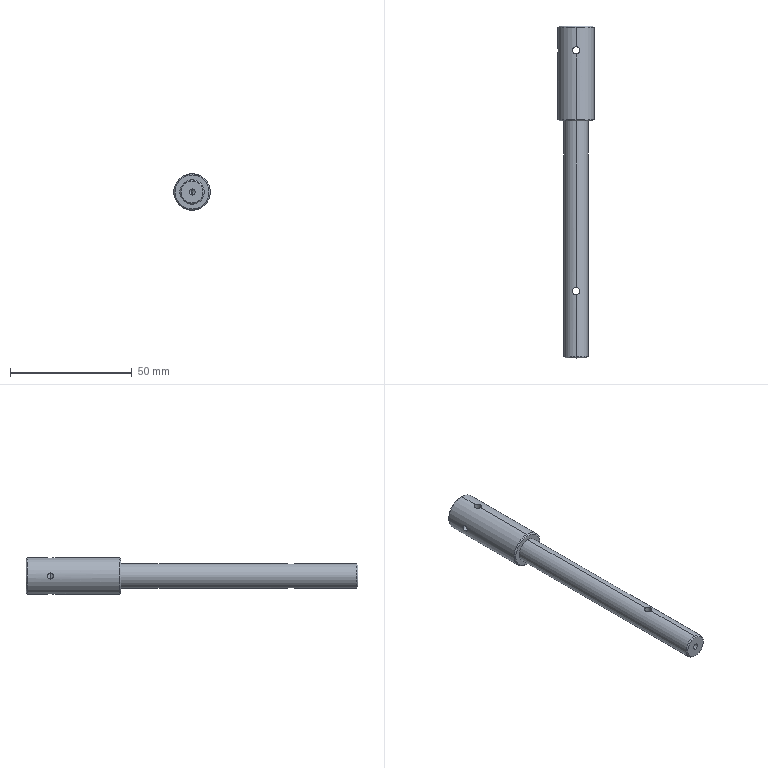Part | SolidWorks | features 3DProfileFeature 3, HoleWzd 3, ICE 2, Chamfer 1, Revolution 1 | 1 solid | 27 faces | box 15 x 136.5 x 15 mm | volume 14219 mm3 | cylinder 14 | cone 10 | plane 3 | commonest cylinder face diameters 2.5 x4 3 x4 3.3 x2 10 x2 15 x2
STEP:
#1=CARTESIAN_POINT('',(0.,-110.5,-5.));
#2=VERTEX_POINT('',#1);
#3=CARTESIAN_POINT('',(-1.5,-109.,-4.77));
#4=VERTEX_POINT('',#3);
#5=CARTESIAN_POINT('',(0.,-110.5,-5.));
#6=CARTESIAN_POINT('',(-0.09847,-110.5,-5.));
#7=CARTESIAN_POINT('',(-0.1985,-110.49,-4.997));
#8=CARTESIAN_POINT('',(-0.3913,-110.451,-4.986));
#9=CARTESIAN_POINT('',(-0.4851,-110.423,-4.977));
#10=CARTESIAN_POINT('',(-0.7586,-110.309,-4.946));
#11=CARTESIAN_POINT('',(-0.9231,-110.198,-4.916));
#12=CARTESIAN_POINT('',(-1.131,-109.991,-4.871));
#13=CARTESIAN_POINT('',(-1.192,-109.916,-4.856));
#14=CARTESIAN_POINT('',(-1.301,-109.753,-4.828));
#15=CARTESIAN_POINT('',(-1.348,-109.666,-4.815));
#16=CARTESIAN_POINT('',(-1.423,-109.485,-4.793));
#17=CARTESIAN_POINT('',(-1.451,-109.391,-4.785));
#18=CARTESIAN_POINT('',(-1.49,-109.198,-4.773));
#19=CARTESIAN_POINT('',(-1.5,-109.098,-4.77));
#20=CARTESIAN_POINT('',(-1.5,-109.,-4.77));
#21=B_SPLINE_CURVE_WITH_KNOTS('',3,(#5,#6,#7,#8,#9,#10,#11,#12,#13,#14,#15,#16,#17,#18,#19,#20),.UNSPECIFIED.,.F.,.F.,(4,2,2,2,2,2,2,4),(0.002359,0.002654,0.002949,0.003538,0.003833,0.004127,0.004422,0.004717),.UNSPECIFIED.);
#22=EDGE_CURVE('',#2,#4,#21,.T.);
#23=ORIENTED_EDGE('',*,*,#22,.T.);
#24=CARTESIAN_POINT('',(-1.5,-109.,4.77));
#25=VERTEX_POINT('',#24);
#26=CARTESIAN_POINT('',(-1.5,-109.,-8.));
#27=DIRECTION('',(0.,0.,1.));
#28=VECTOR('',#27,1000.);
#29=LINE('',#26,#28);
#30=EDGE_CURVE('',#4,#25,#29,.T.);
#31=ORIENTED_EDGE('',*,*,#30,.T.);
#32=CARTESIAN_POINT('',(0.,-110.5,5.));
#33=VERTEX_POINT('',#32);
#34=CARTESIAN_POINT('',(-1.5,-109.,4.77));
#35=CARTESIAN_POINT('',(-1.5,-109.099,4.77));
#36=CARTESIAN_POINT('',(-1.49,-109.197,4.773));
#37=CARTESIAN_POINT('',(-1.452,-109.39,4.785));
#38=CARTESIAN_POINT('',(-1.423,-109.486,4.794));
#39=CARTESIAN_POINT('',(-1.31,-109.757,4.826));
#40=CARTESIAN_POINT('',(-1.198,-109.923,4.856));
#41=CARTESIAN_POINT('',(-0.9923,-110.129,4.901));
#42=CARTESIAN_POINT('',(-0.9158,-110.192,4.916));
#43=CARTESIAN_POINT('',(-0.7532,-110.301,4.944));
#44=CARTESIAN_POINT('',(-0.6674,-110.347,4.956));
#45=CARTESIAN_POINT('',(-0.4865,-110.422,4.977));
#46=CARTESIAN_POINT('',(-0.3907,-110.452,4.986));
#47=CARTESIAN_POINT('',(-0.1978,-110.49,4.997));
#48=CARTESIAN_POINT('',(-0.0997,-110.5,5.));
#49=CARTESIAN_POINT('',(0.,-110.5,5.));
#50=B_SPLINE_CURVE_WITH_KNOTS('',3,(#34,#35,#36,#37,#38,#39,#40,#41,#42,#43,#44,#45,#46,#47,#48,#49),.UNSPECIFIED.,.F.,.F.,(4,2,2,2,2,2,2,4),(0.007075,0.00737,0.007664,0.008254,0.008549,0.008843,0.009138,0.009433),.UNSPECIFIED.);
#51=EDGE_CURVE('',#25,#33,#50,.T.);
#52=ORIENTED_EDGE('',*,*,#51,.T.);
#53=CARTESIAN_POINT('',(1.5,-109.,4.77));
#54=VERTEX_POINT('',#53);
#55=CARTESIAN_POINT('',(0.,-110.5,5.));
#56=CARTESIAN_POINT('',(0.09976,-110.5,5.));
#57=CARTESIAN_POINT('',(0.1977,-110.49,4.997));
#58=CARTESIAN_POINT('',(0.3903,-110.452,4.986));
#59=CARTESIAN_POINT('',(0.4859,-110.423,4.977));
#60=CARTESIAN_POINT('',(0.6674,-110.347,4.956));
#61=CARTESIAN_POINT('',(0.7534,-110.301,4.944));
#62=CARTESIAN_POINT('',(0.916,-110.192,4.916));
#63=CARTESIAN_POINT('',(0.9926,-110.129,4.901));
#64=CARTESIAN_POINT('',(1.199,-109.922,4.856));
#65=CARTESIAN_POINT('',(1.31,-109.756,4.826));
#66=CARTESIAN_POINT('',(1.46,-109.395,4.783));
#67=CARTESIAN_POINT('',(1.5,-109.197,4.77));
#68=CARTESIAN_POINT('',(1.5,-109.,4.77));
#69=B_SPLINE_CURVE_WITH_KNOTS('',3,(#55,#56,#57,#58,#59,#60,#61,#62,#63,#64,#65,#66,#67,#68),.UNSPECIFIED.,.F.,.F.,(4,2,2,2,2,2,4),(0.,0.0002949,0.0005898,0.0008847,0.00118,0.001769,0.002359),.UNSPECIFIED.);
#70=EDGE_CURVE('',#33,#54,#69,.T.);
#71=ORIENTED_EDGE('',*,*,#70,.T.);
#72=CARTESIAN_POINT('',(1.5,-109.,-4.77));
#73=VERTEX_POINT('',#72);
#74=CARTESIAN_POINT('',(1.5,-109.,-8.));
#75=DIRECTION('',(0.,0.,1.));
#76=VECTOR('',#75,1000.);
#77=LINE('',#74,#76);
#78=EDGE_CURVE('',#73,#54,#77,.T.);
#79=ORIENTED_EDGE('',*,*,#78,.F.);
#80=CARTESIAN_POINT('',(1.5,-109.,-4.77));
#81=CARTESIAN_POINT('',(1.5,-109.1,-4.77));
#82=CARTESIAN_POINT('',(1.49,-109.198,-4.773));
#83=CARTESIAN_POINT('',(1.452,-109.39,-4.785));
#84=CARTESIAN_POINT('',(1.423,-109.486,-4.794));
#85=CARTESIAN_POINT('',(1.347,-109.667,-4.815));
#86=CARTESIAN_POINT('',(1.301,-109.753,-4.828));
#87=CARTESIAN_POINT('',(1.192,-109.916,-4.856));
#88=CARTESIAN_POINT('',(1.129,-109.992,-4.871));
#89=CARTESIAN_POINT('',(0.9226,-110.199,-4.916));
#90=CARTESIAN_POINT('',(0.7561,-110.31,-4.946));
#91=CARTESIAN_POINT('',(0.3953,-110.46,-4.988));
#92=CARTESIAN_POINT('',(0.197,-110.5,-5.));
#93=CARTESIAN_POINT('',(0.,-110.5,-5.));
#94=B_SPLINE_CURVE_WITH_KNOTS('',3,(#80,#81,#82,#83,#84,#85,#86,#87,#88,#89,#90,#91,#92,#93),.UNSPECIFIED.,.F.,.F.,(4,2,2,2,2,2,4),(0.,0.0002949,0.0005898,0.0008847,0.00118,0.001769,0.002359),.UNSPECIFIED.);
#95=EDGE_CURVE('',#73,#2,#94,.T.);
#96=ORIENTED_EDGE('',*,*,#95,.T.);
#97=EDGE_LOOP('',(#23,#31,#52,#71,#79,#96));
#98=FACE_OUTER_BOUND('',#97,.T.);
#99=CARTESIAN_POINT('',(0.,-109.,-8.));
#100=DIRECTION('',(0.,0.,1.));
#101=DIRECTION('',(1.,0.,0.));
#102=AXIS2_PLACEMENT_3D('',#99,#100,#101);
#103=CYLINDRICAL_SURFACE('',#102,1.5);
#104=ADVANCED_FACE('',(#98),#103,.F.);
#105=CARTESIAN_POINT('',(-1.5,-10.,-1.25));
#106=VERTEX_POINT('',#105);
#107=CARTESIAN_POINT('',(-1.5,-10.,1.25));
#108=VERTEX_POINT('',#107);
#109=CARTESIAN_POINT('',(-1.5,-10.,-1.25));
#110=CARTESIAN_POINT('',(-1.5,-10.175,-1.25));
#111=CARTESIAN_POINT('',(-1.468,-10.349,-1.212));
#112=CARTESIAN_POINT('',(-1.36,-10.654,-1.078));
#113=CARTESIAN_POINT('',(-1.285,-10.786,-0.9844));
#114=CARTESIAN_POINT('',(-1.125,-11.002,-0.7635));
#115=CARTESIAN_POINT('',(-1.037,-11.088,-0.6353));
#116=CARTESIAN_POINT('',(-0.9263,-11.181,-0.4177));
#117=CARTESIAN_POINT('',(-0.8924,-11.206,-0.3392));
#118=CARTESIAN_POINT('',(-0.8438,-11.241,-0.1749));
#119=CARTESIAN_POINT('',(-0.8291,-11.25,-0.08668));
#120=CARTESIAN_POINT('',(-0.8292,-11.25,0.08724));
#121=CARTESIAN_POINT('',(-0.8439,-11.24,0.1754));
#122=CARTESIAN_POINT('',(-0.8925,-11.206,0.3393));
#123=CARTESIAN_POINT('',(-0.9262,-11.181,0.4175));
#124=CARTESIAN_POINT('',(-1.037,-11.088,0.636));
#125=CARTESIAN_POINT('',(-1.125,-11.001,0.7639));
#126=CARTESIAN_POINT('',(-1.245,-10.839,0.9296));
#127=CARTESIAN_POINT('',(-1.283,-10.78,0.98));
#128=CARTESIAN_POINT('',(-1.354,-10.649,1.071));
#129=CARTESIAN_POINT('',(-1.387,-10.577,1.112));
#130=CARTESIAN_POINT('',(-1.468,-10.35,1.211));
#131=CARTESIAN_POINT('',(-1.5,-10.177,1.25));
#132=CARTESIAN_POINT('',(-1.5,-10.,1.25));
#133=B_SPLINE_CURVE_WITH_KNOTS('',3,(#109,#110,#111,#112,#113,#114,#115,#116,#117,#118,#119,#120,#121,#122,#123,#124,#125,#126,#127,#128,#129,#130,#131,#132),.UNSPECIFIED.,.F.,.F.,(4,2,2,2,2,2,2,2,2,2,2,4),(0.004174,0.004695,0.005216,0.005737,0.005998,0.006258,0.006519,0.006779,0.0073,0.007561,0.007821,0.008342),.UNSPECIFIED.);
#134=EDGE_CURVE('',#106,#108,#133,.T.);
#135=ORIENTED_EDGE('',*,*,#134,.F.);
#136=CARTESIAN_POINT('',(-7.395,-10.,-1.25));
#137=VERTEX_POINT('',#136);
#138=CARTESIAN_POINT('',(-7.5,-10.,-1.25));
#139=DIRECTION('',(-1.,0.,0.));
#140=VECTOR('',#139,1000.);
#141=LINE('',#138,#140);
#142=EDGE_CURVE('',#106,#137,#141,.T.);
#143=ORIENTED_EDGE('',*,*,#142,.T.);
#144=CARTESIAN_POINT('',(-7.395,-10.,1.25));
#145=VERTEX_POINT('',#144);
#146=CARTESIAN_POINT('',(-7.395,-10.,-1.25));
#147=CARTESIAN_POINT('',(-7.395,-10.163,-1.25));
#148=CARTESIAN_POINT('',(-7.401,-10.328,-1.217));
#149=CARTESIAN_POINT('',(-7.42,-10.629,-1.092));
#150=CARTESIAN_POINT('',(-7.434,-10.768,-0.9996));
#151=CARTESIAN_POINT('',(-7.455,-10.941,-0.8269));
#152=CARTESIAN_POINT('',(-7.461,-10.994,-0.7627));
#153=CARTESIAN_POINT('',(-7.474,-11.084,-0.6272));
#154=CARTESIAN_POINT('',(-7.48,-11.123,-0.5555));
#155=CARTESIAN_POINT('',(-7.494,-11.217,-0.3283));
#156=CARTESIAN_POINT('',(-7.5,-11.25,-0.1659));
#157=CARTESIAN_POINT('',(-7.5,-11.25,0.1644));
#158=CARTESIAN_POINT('',(-7.494,-11.217,0.3271));
#159=CARTESIAN_POINT('',(-7.475,-11.092,0.6295));
#160=CARTESIAN_POINT('',(-7.461,-10.999,0.7682));
#161=CARTESIAN_POINT('',(-7.434,-10.77,0.9984));
#162=CARTESIAN_POINT('',(-7.42,-10.63,1.092));
#163=CARTESIAN_POINT('',(-7.401,-10.33,1.217));
#164=CARTESIAN_POINT('',(-7.395,-10.165,1.25));
#165=CARTESIAN_POINT('',(-7.395,-10.,1.25));
#166=B_SPLINE_CURVE_WITH_KNOTS('',3,(#146,#147,#148,#149,#150,#151,#152,#153,#154,#155,#156,#157,#158,#159,#160,#161,#162,#163,#164,#165),.UNSPECIFIED.,.F.,.F.,(4,2,2,2,2,2,2,2,2,4),(0.003915,0.004404,0.004893,0.005138,0.005383,0.005872,0.006361,0.00685,0.00734,0.007829),.UNSPECIFIED.);
#167=EDGE_CURVE('',#137,#145,#166,.T.);
#168=ORIENTED_EDGE('',*,*,#167,.T.);
#169=CARTESIAN_POINT('',(-7.5,-10.,1.25));
#170=DIRECTION('',(-1.,0.,0.));
#171=VECTOR('',#170,1000.);
#172=LINE('',#169,#171);
#173=EDGE_CURVE('',#108,#145,#172,.T.);
#174=ORIENTED_EDGE('',*,*,#173,.F.);
#175=EDGE_LOOP('',(#135,#143,#168,#174));
#176=FACE_OUTER_BOUND('',#175,.T.);
#177=CARTESIAN_POINT('',(-7.5,-10.,0.));
#178=DIRECTION('',(-1.,0.,0.));
#179=DIRECTION('',(0.,0.,1.));
#180=AXIS2_PLACEMENT_3D('',#177,#178,#179);
#181=CYLINDRICAL_SURFACE('',#180,1.25);
#182=ADVANCED_FACE('',(#176),#181,.F.);
#183=CARTESIAN_POINT('',(0.,-136.5,-4.5));
#184=VERTEX_POINT('',#183);
#185=CARTESIAN_POINT('',(0.,-136.5,4.5));
#186=VERTEX_POINT('',#185);
#187=CARTESIAN_POINT('',(0.,-136.5,0.));
#188=DIRECTION('',(0.,-1.,0.));
#189=DIRECTION('',(0.,0.,-1.));
#190=AXIS2_PLACEMENT_3D('',#187,#188,#189);
#191=CIRCLE('',#190,4.5);
#192=EDGE_CURVE('',#184,#186,#191,.T.);
#193=ORIENTED_EDGE('',*,*,#192,.F.);
#194=CARTESIAN_POINT('',(0.,-136.,-5.));
#195=VERTEX_POINT('',#194);
#196=CARTESIAN_POINT('',(0.,-136.,-5.));
#197=DIRECTION('',(0.,0.7071,-0.7071));
#198=VECTOR('',#197,1000.);
#199=LINE('',#196,#198);
#200=EDGE_CURVE('',#184,#195,#199,.T.);
#201=ORIENTED_EDGE('',*,*,#200,.T.);
#202=CARTESIAN_POINT('',(0.,-136.,5.));
#203=VERTEX_POINT('',#202);
#204=CARTESIAN_POINT('',(0.,-136.,0.));
#205=DIRECTION('',(0.,1.,0.));
#206=DIRECTION('',(0.,0.,-1.));
#207=AXIS2_PLACEMENT_3D('',#204,#205,#206);
#208=CIRCLE('',#207,5.);
#209=EDGE_CURVE('',#203,#195,#208,.T.);
#210=ORIENTED_EDGE('',*,*,#209,.F.);
#211=CARTESIAN_POINT('',(0.,-136.,5.));
#212=DIRECTION('',(0.,0.7071,0.7071));
#213=VECTOR('',#212,1000.);
#214=LINE('',#211,#213);
#215=EDGE_CURVE('',#186,#203,#214,.T.);
#216=ORIENTED_EDGE('',*,*,#215,.F.);
#217=EDGE_LOOP('',(#193,#201,#210,#216));
#218=FACE_OUTER_BOUND('',#217,.T.);
#219=CARTESIAN_POINT('',(0.,-136.,0.));
#220=DIRECTION('',(0.,1.,0.));
#221=DIRECTION('',(0.,0.,1.));
#222=AXIS2_PLACEMENT_3D('',#219,#220,#221);
#223=CONICAL_SURFACE('',#222,5.,0.7854);
#224=ADVANCED_FACE('',(#218),#223,.T.);
#225=CARTESIAN_POINT('',(0.,-39.,-7.));
#226=VERTEX_POINT('',#225);
#227=CARTESIAN_POINT('',(0.,-39.,7.));
#228=VERTEX_POINT('',#227);
#229=CARTESIAN_POINT('',(0.,-39.,0.));
#230=DIRECTION('',(0.,-1.,0.));
#231=DIRECTION('',(0.,0.,-1.));
#232=AXIS2_PLACEMENT_3D('',#229,#230,#231);
#233=CIRCLE('',#232,7.);
#234=EDGE_CURVE('',#226,#228,#233,.T.);
#235=ORIENTED_EDGE('',*,*,#234,.F.);
#236=CARTESIAN_POINT('',(0.,-38.5,-7.5));
#237=VERTEX_POINT('',#236);
#238=CARTESIAN_POINT('',(0.,-38.5,-7.5));
#239=DIRECTION('',(0.,0.7071,-0.7071));
#240=VECTOR('',#239,1000.);
#241=LINE('',#238,#240);
#242=EDGE_CURVE('',#226,#237,#241,.T.);
#243=ORIENTED_EDGE('',*,*,#242,.T.);
#244=CARTESIAN_POINT('',(0.,-38.5,7.5));
#245=VERTEX_POINT('',#244);
#246=CARTESIAN_POINT('',(0.,-38.5,0.));
#247=DIRECTION('',(0.,1.,0.));
#248=DIRECTION('',(0.,0.,-1.));
#249=AXIS2_PLACEMENT_3D('',#246,#247,#248);
#250=CIRCLE('',#249,7.5);
#251=EDGE_CURVE('',#245,#237,#250,.T.);
#252=ORIENTED_EDGE('',*,*,#251,.F.);
#253=CARTESIAN_POINT('',(0.,-38.5,7.5));
#254=DIRECTION('',(0.,0.7071,0.7071));
#255=VECTOR('',#254,1000.);
#256=LINE('',#253,#255);
#257=EDGE_CURVE('',#228,#245,#256,.T.);
#258=ORIENTED_EDGE('',*,*,#257,.F.);
#259=EDGE_LOOP('',(#235,#243,#252,#258));
#260=FACE_OUTER_BOUND('',#259,.T.);
#261=CARTESIAN_POINT('',(0.,-38.5,0.));
#262=DIRECTION('',(0.,1.,0.));
#263=DIRECTION('',(0.,0.,1.));
#264=AXIS2_PLACEMENT_3D('',#261,#262,#263);
#265=CONICAL_SURFACE('',#264,7.5,0.7854);
#266=ADVANCED_FACE('',(#260),#265,.T.);
#267=CARTESIAN_POINT('',(0.,0.,7.));
#268=VERTEX_POINT('',#267);
#269=CARTESIAN_POINT('',(0.,0.,-7.));
#270=VERTEX_POINT('',#269);
#271=CARTESIAN_POINT('',(0.,0.,0.));
#272=DIRECTION('',(0.,1.,0.));
#273=DIRECTION('',(0.,0.,1.));
#274=AXIS2_PLACEMENT_3D('',#271,#272,#273);
#275=CIRCLE('',#274,7.);
#276=EDGE_CURVE('',#268,#270,#275,.T.);
#277=ORIENTED_EDGE('',*,*,#276,.F.);
#278=CARTESIAN_POINT('',(0.,-0.5,7.5));
#279=VERTEX_POINT('',#278);
#280=CARTESIAN_POINT('',(0.,0.,7.));
#281=DIRECTION('',(0.,-0.7071,0.7071));
#282=VECTOR('',#281,1000.);
#283=LINE('',#280,#282);
#284=EDGE_CURVE('',#268,#279,#283,.T.);
#285=ORIENTED_EDGE('',*,*,#284,.T.);
#286=CARTESIAN_POINT('',(0.,-0.5,-7.5));
#287=VERTEX_POINT('',#286);
#288=CARTESIAN_POINT('',(0.,-0.5,0.));
#289=DIRECTION('',(0.,-1.,0.));
#290=DIRECTION('',(0.,0.,1.));
#291=AXIS2_PLACEMENT_3D('',#288,#289,#290);
#292=CIRCLE('',#291,7.5);
#293=EDGE_CURVE('',#287,#279,#292,.T.);
#294=ORIENTED_EDGE('',*,*,#293,.F.);
#295=CARTESIAN_POINT('',(0.,0.,-7.));
#296=DIRECTION('',(0.,-0.7071,-0.7071));
#297=VECTOR('',#296,1000.);
#298=LINE('',#295,#297);
#299=EDGE_CURVE('',#270,#287,#298,.T.);
#300=ORIENTED_EDGE('',*,*,#299,.F.);
#301=EDGE_LOOP('',(#277,#285,#294,#300));
#302=FACE_OUTER_BOUND('',#301,.T.);
#303=CARTESIAN_POINT('',(0.,0.,0.));
#304=DIRECTION('',(0.,-1.,0.));
#305=DIRECTION('',(0.,0.,-1.));
#306=AXIS2_PLACEMENT_3D('',#303,#304,#305);
#307=CONICAL_SURFACE('',#306,7.,0.7854);
#308=ADVANCED_FACE('',(#302),#307,.T.);
#309=CARTESIAN_POINT('',(0.,-129.,1.25));
#310=VERTEX_POINT('',#309);
#311=CARTESIAN_POINT('',(0.,-129.,-1.25));
#312=VERTEX_POINT('',#311);
#313=CARTESIAN_POINT('',(0.,-129.,0.));
#314=DIRECTION('',(0.,-1.,0.));
#315=DIRECTION('',(0.,0.,-1.));
#316=AXIS2_PLACEMENT_3D('',#313,#314,#315);
#317=CIRCLE('',#316,1.25);
#318=EDGE_CURVE('',#310,#312,#317,.T.);
#319=ORIENTED_EDGE('',*,*,#318,.F.);
#320=CARTESIAN_POINT('',(0.,-136.5,1.25));
#321=VERTEX_POINT('',#320);
#322=CARTESIAN_POINT('',(0.,-136.5,1.25));
#323=DIRECTION('',(0.,-1.,0.));
#324=VECTOR('',#323,1000.);
#325=LINE('',#322,#324);
#326=EDGE_CURVE('',#310,#321,#325,.T.);
#327=ORIENTED_EDGE('',*,*,#326,.T.);
#328=CARTESIAN_POINT('',(0.,-136.5,-1.25));
#329=VERTEX_POINT('',#328);
#330=CARTESIAN_POINT('',(0.,-136.5,0.));
#331=DIRECTION('',(0.,-1.,0.));
#332=DIRECTION('',(0.,0.,-1.));
#333=AXIS2_PLACEMENT_3D('',#330,#331,#332);
#334=CIRCLE('',#333,1.25);
#335=EDGE_CURVE('',#321,#329,#334,.T.);
#336=ORIENTED_EDGE('',*,*,#335,.T.);
#337=CARTESIAN_POINT('',(0.,-136.5,-1.25));
#338=DIRECTION('',(0.,-1.,0.));
#339=VECTOR('',#338,1000.);
#340=LINE('',#337,#339);
#341=EDGE_CURVE('',#312,#329,#340,.T.);
#342=ORIENTED_EDGE('',*,*,#341,.F.);
#343=EDGE_LOOP('',(#319,#327,#336,#342));
#344=FACE_OUTER_BOUND('',#343,.T.);
#345=CARTESIAN_POINT('',(0.,-136.5,0.));
#346=DIRECTION('',(0.,-1.,0.));
#347=DIRECTION('',(0.,0.,-1.));
#348=AXIS2_PLACEMENT_3D('',#345,#346,#347);
#349=CYLINDRICAL_SURFACE('',#348,1.25);
#350=ADVANCED_FACE('',(#344),#349,.F.);
#351=CARTESIAN_POINT('',(0.,-128.249,0.));
#352=VERTEX_POINT('',#351);
#353=CARTESIAN_POINT('',(0.,-129.,-1.25));
#354=DIRECTION('',(0.,-0.515,-0.8572));
#355=VECTOR('',#354,1000.);
#356=LINE('',#353,#355);
#357=EDGE_CURVE('',#352,#312,#356,.T.);
#358=ORIENTED_EDGE('',*,*,#357,.F.);
#359=CARTESIAN_POINT('',(0.,-129.,1.25));
#360=DIRECTION('',(0.,-0.515,0.8572));
#361=VECTOR('',#360,1000.);
#362=LINE('',#359,#361);
#363=EDGE_CURVE('',#352,#310,#362,.T.);
#364=ORIENTED_EDGE('',*,*,#363,.T.);
#365=ORIENTED_EDGE('',*,*,#318,.T.);
#366=EDGE_LOOP('',(#358,#364,#365));
#367=FACE_OUTER_BOUND('',#366,.T.);
#368=CARTESIAN_POINT('',(0.,-129.,0.));
#369=DIRECTION('',(0.,-1.,0.));
#370=DIRECTION('',(0.,0.,-1.));
#371=AXIS2_PLACEMENT_3D('',#368,#369,#370);
#372=CONICAL_SURFACE('',#371,1.25,1.03);
#373=ADVANCED_FACE('',(#367),#372,.F.);
#374=CARTESIAN_POINT('',(0.,-11.5,-7.5));
#375=VERTEX_POINT('',#374);
#376=CARTESIAN_POINT('',(-1.5,-10.,-7.348));
#377=VERTEX_POINT('',#376);
#378=CARTESIAN_POINT('',(0.,-11.5,-7.5));
#379=CARTESIAN_POINT('',(-0.09809,-11.5,-7.5));
#380=CARTESIAN_POINT('',(-0.1978,-11.49,-7.498));
#381=CARTESIAN_POINT('',(-0.3903,-11.452,-7.49));
#382=CARTESIAN_POINT('',(-0.4839,-11.423,-7.485));
#383=CARTESIAN_POINT('',(-0.7567,-11.31,-7.464));
#384=CARTESIAN_POINT('',(-0.9216,-11.2,-7.444));
#385=CARTESIAN_POINT('',(-1.131,-10.991,-7.415));
#386=CARTESIAN_POINT('',(-1.192,-10.915,-7.405));
#387=CARTESIAN_POINT('',(-1.301,-10.753,-7.386));
#388=CARTESIAN_POINT('',(-1.348,-10.665,-7.378));
#389=CARTESIAN_POINT('',(-1.423,-10.484,-7.364));
#390=CARTESIAN_POINT('',(-1.452,-10.39,-7.358));
#391=CARTESIAN_POINT('',(-1.49,-10.198,-7.35));
#392=CARTESIAN_POINT('',(-1.5,-10.098,-7.348));
#393=CARTESIAN_POINT('',(-1.5,-10.,-7.348));
#394=B_SPLINE_CURVE_WITH_KNOTS('',3,(#378,#379,#380,#381,#382,#383,#384,#385,#386,#387,#388,#389,#390,#391,#392,#393),.UNSPECIFIED.,.F.,.F.,(4,2,2,2,2,2,2,4),(0.002351,0.002645,0.002939,0.003526,0.00382,0.004114,0.004408,0.004702),.UNSPECIFIED.);
#395=EDGE_CURVE('',#375,#377,#394,.T.);
#396=ORIENTED_EDGE('',*,*,#395,.T.);
#397=CARTESIAN_POINT('',(-1.5,-10.,-8.));
#398=DIRECTION('',(0.,0.,1.));
#399=VECTOR('',#398,1000.);
#400=LINE('',#397,#399);
#401=EDGE_CURVE('',#377,#106,#400,.T.);
#402=ORIENTED_EDGE('',*,*,#401,.T.);
#403=ORIENTED_EDGE('',*,*,#134,.T.);
#404=CARTESIAN_POINT('',(-1.5,-10.,7.348));
#405=VERTEX_POINT('',#404);
#406=CARTESIAN_POINT('',(-1.5,-10.,-8.));
#407=DIRECTION('',(0.,0.,1.));
#408=VECTOR('',#407,1000.);
#409=LINE('',#406,#408);
#410=EDGE_CURVE('',#108,#405,#409,.T.);
#411=ORIENTED_EDGE('',*,*,#410,.T.);
#412=CARTESIAN_POINT('',(0.,-11.5,7.5));
#413=VERTEX_POINT('',#412);
#414=CARTESIAN_POINT('',(-1.5,-10.,7.348));
#415=CARTESIAN_POINT('',(-1.5,-10.099,7.348));
#416=CARTESIAN_POINT('',(-1.49,-10.197,7.35));
#417=CARTESIAN_POINT('',(-1.452,-10.389,7.358));
#418=CARTESIAN_POINT('',(-1.423,-10.484,7.364));
#419=CARTESIAN_POINT('',(-1.31,-10.756,7.385));
#420=CARTESIAN_POINT('',(-1.199,-10.922,7.405));
#421=CARTESIAN_POINT('',(-0.9233,-11.198,7.444));
#422=CARTESIAN_POINT('',(-0.7565,-11.31,7.464));
#423=CARTESIAN_POINT('',(-0.3958,-11.46,7.492));
#424=CARTESIAN_POINT('',(-0.1986,-11.5,7.5));
#425=CARTESIAN_POINT('',(0.,-11.5,7.5));
#426=B_SPLINE_CURVE_WITH_KNOTS('',3,(#414,#415,#416,#417,#418,#419,#420,#421,#422,#423,#424,#425),.UNSPECIFIED.,.F.,.F.,(4,2,2,2,2,4),(0.007052,0.007346,0.00764,0.008227,0.008815,0.009402),.UNSPECIFIED.);
#427=EDGE_CURVE('',#405,#413,#426,.T.);
#428=ORIENTED_EDGE('',*,*,#427,.T.);
#429=CARTESIAN_POINT('',(1.5,-10.,7.348));
#430=VERTEX_POINT('',#429);
#431=CARTESIAN_POINT('',(0.,-11.5,7.5));
#432=CARTESIAN_POINT('',(0.0994,-11.5,7.5));
#433=CARTESIAN_POINT('',(0.1971,-11.49,7.498));
#434=CARTESIAN_POINT('',(0.3892,-11.452,7.491));
#435=CARTESIAN_POINT('',(0.4847,-11.423,7.485));
#436=CARTESIAN_POINT('',(0.6662,-11.348,7.471));
#437=CARTESIAN_POINT('',(0.7523,-11.301,7.463));
#438=CARTESIAN_POINT('',(0.9152,-11.192,7.444));
#439=CARTESIAN_POINT('',(0.9921,-11.129,7.434));
#440=CARTESIAN_POINT('',(1.199,-10.922,7.405));
#441=CARTESIAN_POINT('',(1.311,-10.755,7.385));
#442=CARTESIAN_POINT('',(1.46,-10.394,7.357));
#443=CARTESIAN_POINT('',(1.5,-10.196,7.348));
#444=CARTESIAN_POINT('',(1.5,-10.,7.348));
#445=B_SPLINE_CURVE_WITH_KNOTS('',3,(#431,#432,#433,#434,#435,#436,#437,#438,#439,#440,#441,#442,#443,#444),.UNSPECIFIED.,.F.,.F.,(4,2,2,2,2,2,4),(0.,0.0002939,0.0005878,0.0008818,0.001176,0.001764,0.002351),.UNSPECIFIED.);
#446=EDGE_CURVE('',#413,#430,#445,.T.);
#447=ORIENTED_EDGE('',*,*,#446,.T.);
#448=CARTESIAN_POINT('',(1.5,-10.,-7.348));
#449=VERTEX_POINT('',#448);
#450=CARTESIAN_POINT('',(1.5,-10.,-8.));
#451=DIRECTION('',(0.,0.,1.));
#452=VECTOR('',#451,1000.);
#453=LINE('',#450,#452);
#454=EDGE_CURVE('',#449,#430,#453,.T.);
#455=ORIENTED_EDGE('',*,*,#454,.F.);
#456=CARTESIAN_POINT('',(1.5,-10.,-7.348));
#457=CARTESIAN_POINT('',(1.5,-10.099,-7.348));
#458=CARTESIAN_POINT('',(1.49,-10.197,-7.35));
#459=CARTESIAN_POINT('',(1.452,-10.389,-7.358));
#460=CARTESIAN_POINT('',(1.423,-10.485,-7.364));
#461=CARTESIAN_POINT('',(1.348,-10.666,-7.378));
#462=CARTESIAN_POINT('',(1.301,-10.752,-7.386));
#463=CARTESIAN_POINT('',(1.192,-10.915,-7.405));
#464=CARTESIAN_POINT('',(1.129,-10.992,-7.415));
#465=CARTESIAN_POINT('',(0.9221,-11.199,-7.444));
#466=CARTESIAN_POINT('',(0.7551,-11.311,-7.464));
#467=CARTESIAN_POINT('',(0.3941,-11.46,-7.492));
#468=CARTESIAN_POINT('',(0.1963,-11.5,-7.5));
#469=CARTESIAN_POINT('',(0.,-11.5,-7.5));
#470=B_SPLINE_CURVE_WITH_KNOTS('',3,(#456,#457,#458,#459,#460,#461,#462,#463,#464,#465,#466,#467,#468,#469),.UNSPECIFIED.,.F.,.F.,(4,2,2,2,2,2,4),(0.,0.0002939,0.0005878,0.0008818,0.001176,0.001764,0.002351),.UNSPECIFIED.);
#471=EDGE_CURVE('',#449,#375,#470,.T.);
#472=ORIENTED_EDGE('',*,*,#471,.T.);
#473=EDGE_LOOP('',(#396,#402,#403,#411,#428,#447,#455,#472));
#474=FACE_OUTER_BOUND('',#473,.T.);
#475=CARTESIAN_POINT('',(0.,-10.,-8.));
#476=DIRECTION('',(0.,0.,1.));
#477=DIRECTION('',(1.,0.,0.));
#478=AXIS2_PLACEMENT_3D('',#475,#476,#477);
#479=CYLINDRICAL_SURFACE('',#478,1.5);
#480=ADVANCED_FACE('',(#474),#479,.F.);
#481=CARTESIAN_POINT('',(0.,-8.1,-1.65));
#482=VERTEX_POINT('',#481);
#483=CARTESIAN_POINT('',(0.,-8.1,1.65));
#484=VERTEX_POINT('',#483);
#485=CARTESIAN_POINT('',(0.,-8.1,0.));
#486=DIRECTION('',(0.,1.,0.));
#487=DIRECTION('',(0.,0.,1.));
#488=AXIS2_PLACEMENT_3D('',#485,#486,#487);
#489=CIRCLE('',#488,1.65);
#490=EDGE_CURVE('',#482,#484,#489,.T.);
#491=ORIENTED_EDGE('',*,*,#490,.F.);
#492=CARTESIAN_POINT('',(0.,0.,-1.65));
#493=VERTEX_POINT('',#492);
#494=CARTESIAN_POINT('',(0.,0.,-1.65));
#495=DIRECTION('',(0.,1.,0.));
#496=VECTOR('',#495,1000.);
#497=LINE('',#494,#496);
#498=EDGE_CURVE('',#482,#493,#497,.T.);
#499=ORIENTED_EDGE('',*,*,#498,.T.);
#500=CARTESIAN_POINT('',(0.,0.,1.65));
#501=VERTEX_POINT('',#500);
#502=CARTESIAN_POINT('',(0.,0.,0.));
#503=DIRECTION('',(0.,1.,0.));
#504=DIRECTION('',(0.,0.,1.));
#505=AXIS2_PLACEMENT_3D('',#502,#503,#504);
#506=CIRCLE('',#505,1.65);
#507=EDGE_CURVE('',#493,#501,#506,.T.);
#508=ORIENTED_EDGE('',*,*,#507,.T.);
#509=CARTESIAN_POINT('',(0.,0.,1.65));
#510=DIRECTION('',(0.,1.,0.));
#511=VECTOR('',#510,1000.);
#512=LINE('',#509,#511);
#513=EDGE_CURVE('',#484,#501,#512,.T.);
#514=ORIENTED_EDGE('',*,*,#513,.F.);
#515=EDGE_LOOP('',(#491,#499,#508,#514));
#516=FACE_OUTER_BOUND('',#515,.T.);
#517=CARTESIAN_POINT('',(0.,0.,0.));
#518=DIRECTION('',(0.,1.,0.));
#519=DIRECTION('',(0.,0.,1.));
#520=AXIS2_PLACEMENT_3D('',#517,#518,#519);
#521=CYLINDRICAL_SURFACE('',#520,1.65);
#522=ADVANCED_FACE('',(#516),#521,.F.);
#523=CARTESIAN_POINT('',(0.,-8.5,0.9843));
#524=VERTEX_POINT('',#523);
#525=CARTESIAN_POINT('',(0.,-8.5,-0.9843));
#526=VERTEX_POINT('',#525);
#527=CARTESIAN_POINT('',(0.,-8.5,0.9843));
#528=CARTESIAN_POINT('',(-0.1125,-8.5,0.9843));
#529=CARTESIAN_POINT('',(-0.2218,-8.514,0.9415));
#530=CARTESIAN_POINT('',(-0.4001,-8.551,0.8115));
#531=CARTESIAN_POINT('',(-0.472,-8.575,0.7258));
#532=CARTESIAN_POINT('',(-0.6414,-8.639,0.446));
#533=CARTESIAN_POINT('',(-0.6979,-8.672,0.2215));
#534=CARTESIAN_POINT('',(-0.6977,-8.672,-0.1121));
#535=CARTESIAN_POINT('',(-0.6835,-8.664,-0.2227));
#536=CARTESIAN_POINT('',(-0.6267,-8.637,-0.4374));
#537=CARTESIAN_POINT('',(-0.5854,-8.618,-0.5384));
#538=CARTESIAN_POINT('',(-0.4715,-8.575,-0.7266));
#539=CARTESIAN_POINT('',(-0.3996,-8.551,-0.812));
#540=CARTESIAN_POINT('',(-0.2213,-8.514,-0.9418));
#541=CARTESIAN_POINT('',(-0.1127,-8.5,-0.9843));
#542=CARTESIAN_POINT('',(0.,-8.5,-0.9843));
#543=B_SPLINE_CURVE_WITH_KNOTS('',3,(#527,#528,#529,#530,#531,#532,#533,#534,#535,#536,#537,#538,#539,#540,#541,#542),.UNSPECIFIED.,.F.,.F.,(4,2,2,2,2,2,2,4),(0.00285,0.003185,0.00352,0.00419,0.004525,0.00486,0.005195,0.00553),.UNSPECIFIED.);
#544=EDGE_CURVE('',#524,#526,#543,.T.);
#545=ORIENTED_EDGE('',*,*,#544,.T.);
#546=CARTESIAN_POINT('',(0.,-8.1,-1.65));
#547=DIRECTION('',(0.,0.515,-0.8572));
#548=VECTOR('',#547,1000.);
#549=LINE('',#546,#548);
#550=EDGE_CURVE('',#526,#482,#549,.T.);
#551=ORIENTED_EDGE('',*,*,#550,.T.);
#552=ORIENTED_EDGE('',*,*,#490,.T.);
#553=CARTESIAN_POINT('',(0.,-8.1,1.65));
#554=DIRECTION('',(0.,0.515,0.8572));
#555=VECTOR('',#554,1000.);
#556=LINE('',#553,#555);
#557=EDGE_CURVE('',#524,#484,#556,.T.);
#558=ORIENTED_EDGE('',*,*,#557,.F.);
#559=EDGE_LOOP('',(#545,#551,#552,#558));
#560=FACE_OUTER_BOUND('',#559,.T.);
#561=CARTESIAN_POINT('',(0.,-8.1,0.));
#562=DIRECTION('',(0.,1.,0.));
#563=DIRECTION('',(0.,0.,1.));
#564=AXIS2_PLACEMENT_3D('',#561,#562,#563);
#565=CONICAL_SURFACE('',#564,1.65,1.03);
#566=ADVANCED_FACE('',(#560),#565,.F.);
#567=ORIENTED_EDGE('',*,*,#209,.T.);
#568=CARTESIAN_POINT('',(0.,0.,-5.));
#569=DIRECTION('',(0.,1.,0.));
#570=VECTOR('',#569,1000.);
#571=LINE('',#568,#570);
#572=EDGE_CURVE('',#195,#2,#571,.T.);
#573=ORIENTED_EDGE('',*,*,#572,.T.);
#574=ORIENTED_EDGE('',*,*,#95,.F.);
#575=CARTESIAN_POINT('',(0.,-107.5,-5.));
#576=VERTEX_POINT('',#575);
#577=CARTESIAN_POINT('',(0.,-107.5,-5.));
#578=CARTESIAN_POINT('',(0.09885,-107.5,-5.));
#579=CARTESIAN_POINT('',(0.1966,-107.51,-4.997));
#580=CARTESIAN_POINT('',(0.3899,-107.548,-4.986));
#581=CARTESIAN_POINT('',(0.4856,-107.577,-4.977));
#582=CARTESIAN_POINT('',(0.7566,-107.69,-4.946));
#583=CARTESIAN_POINT('',(0.9229,-107.802,-4.916));
#584=CARTESIAN_POINT('',(1.129,-108.008,-4.871));
#585=CARTESIAN_POINT('',(1.192,-108.084,-4.856));
#586=CARTESIAN_POINT('',(1.301,-108.247,-4.828));
#587=CARTESIAN_POINT('',(1.347,-108.333,-4.815));
#588=CARTESIAN_POINT('',(1.422,-108.514,-4.794));
#589=CARTESIAN_POINT('',(1.452,-108.609,-4.785));
#590=CARTESIAN_POINT('',(1.49,-108.802,-4.773));
#591=CARTESIAN_POINT('',(1.5,-108.9,-4.77));
#592=CARTESIAN_POINT('',(1.5,-109.,-4.77));
#593=B_SPLINE_CURVE_WITH_KNOTS('',3,(#577,#578,#579,#580,#581,#582,#583,#584,#585,#586,#587,#588,#589,#590,#591,#592),.UNSPECIFIED.,.F.,.F.,(4,2,2,2,2,2,2,4),(0.007075,0.00737,0.007664,0.008254,0.008548,0.008843,0.009138,0.009433),.UNSPECIFIED.);
#594=EDGE_CURVE('',#576,#73,#593,.T.);
#595=ORIENTED_EDGE('',*,*,#594,.F.);
#596=CARTESIAN_POINT('',(0.,-39.,-5.));
#597=VERTEX_POINT('',#596);
#598=CARTESIAN_POINT('',(0.,0.,-5.));
#599=DIRECTION('',(0.,1.,0.));
#600=VECTOR('',#599,1000.);
#601=LINE('',#598,#600);
#602=EDGE_CURVE('',#576,#597,#601,.T.);
#603=ORIENTED_EDGE('',*,*,#602,.T.);
#604=CARTESIAN_POINT('',(0.,-39.,5.));
#605=VERTEX_POINT('',#604);
#606=CARTESIAN_POINT('',(0.,-39.,0.));
#607=DIRECTION('',(0.,1.,0.));
#608=DIRECTION('',(0.,0.,1.));
#609=AXIS2_PLACEMENT_3D('',#606,#607,#608);
#610=CIRCLE('',#609,5.);
#611=EDGE_CURVE('',#605,#597,#610,.T.);
#612=ORIENTED_EDGE('',*,*,#611,.F.);
#613=CARTESIAN_POINT('',(0.,-107.5,5.));
#614=VERTEX_POINT('',#613);
#615=CARTESIAN_POINT('',(0.,0.,5.));
#616=DIRECTION('',(0.,1.,0.));
#617=VECTOR('',#616,1000.);
#618=LINE('',#615,#617);
#619=EDGE_CURVE('',#614,#605,#618,.T.);
#620=ORIENTED_EDGE('',*,*,#619,.F.);
#621=CARTESIAN_POINT('',(1.5,-109.,4.77));
#622=CARTESIAN_POINT('',(1.5,-108.902,4.77));
#623=CARTESIAN_POINT('',(1.49,-108.802,4.773));
#624=CARTESIAN_POINT('',(1.451,-108.609,4.785));
#625=CARTESIAN_POINT('',(1.423,-108.515,4.793));
#626=CARTESIAN_POINT('',(1.309,-108.242,4.826));
#627=CARTESIAN_POINT('',(1.199,-108.077,4.856));
#628=CARTESIAN_POINT('',(0.9908,-107.87,4.901));
#629=CARTESIAN_POINT('',(0.9157,-107.808,4.916));
#630=CARTESIAN_POINT('',(0.7536,-107.699,4.944));
#631=CARTESIAN_POINT('',(0.6658,-107.652,4.956));
#632=CARTESIAN_POINT('',(0.485,-107.577,4.977));
#633=CARTESIAN_POINT('',(0.3915,-107.549,4.986));
#634=CARTESIAN_POINT('',(0.1977,-107.51,4.997));
#635=CARTESIAN_POINT('',(0.09824,-107.5,5.));
#636=CARTESIAN_POINT('',(0.,-107.5,5.));
#637=B_SPLINE_CURVE_WITH_KNOTS('',3,(#621,#622,#623,#624,#625,#626,#627,#628,#629,#630,#631,#632,#633,#634,#635,#636),.UNSPECIFIED.,.F.,.F.,(4,2,2,2,2,2,2,4),(0.002359,0.002654,0.002949,0.003538,0.003833,0.004128,0.004422,0.004717),.UNSPECIFIED.);
#638=EDGE_CURVE('',#54,#614,#637,.T.);
#639=ORIENTED_EDGE('',*,*,#638,.F.);
#640=ORIENTED_EDGE('',*,*,#70,.F.);
#641=CARTESIAN_POINT('',(0.,0.,5.));
#642=DIRECTION('',(0.,1.,0.));
#643=VECTOR('',#642,1000.);
#644=LINE('',#641,#643);
#645=EDGE_CURVE('',#203,#33,#644,.T.);
#646=ORIENTED_EDGE('',*,*,#645,.F.);
#647=EDGE_LOOP('',(#567,#573,#574,#595,#603,#612,#620,#639,#640,#646));
#648=FACE_OUTER_BOUND('',#647,.T.);
#649=CARTESIAN_POINT('',(0.,0.,0.));
#650=DIRECTION('',(0.,1.,0.));
#651=DIRECTION('',(0.,0.,1.));
#652=AXIS2_PLACEMENT_3D('',#649,#650,#651);
#653=CYLINDRICAL_SURFACE('',#652,5.);
#654=ADVANCED_FACE('',(#648),#653,.T.);
#655=ORIENTED_EDGE('',*,*,#251,.T.);
#656=CARTESIAN_POINT('',(0.,0.,-7.5));
#657=DIRECTION('',(0.,1.,0.));
#658=VECTOR('',#657,1000.);
#659=LINE('',#656,#658);
#660=EDGE_CURVE('',#237,#375,#659,.T.);
#661=ORIENTED_EDGE('',*,*,#660,.T.);
#662=ORIENTED_EDGE('',*,*,#471,.F.);
#663=CARTESIAN_POINT('',(0.,-8.5,-7.5));
#664=VERTEX_POINT('',#663);
#665=CARTESIAN_POINT('',(0.,-8.5,-7.5));
#666=CARTESIAN_POINT('',(0.09899,-8.5,-7.5));
#667=CARTESIAN_POINT('',(0.1965,-8.51,-7.498));
#668=CARTESIAN_POINT('',(0.3887,-8.548,-7.491));
#669=CARTESIAN_POINT('',(0.4843,-8.577,-7.485));
#670=CARTESIAN_POINT('',(0.7559,-8.69,-7.464));
#671=CARTESIAN_POINT('',(0.9224,-8.801,-7.444));
#672=CARTESIAN_POINT('',(1.198,-9.077,-7.405));
#673=CARTESIAN_POINT('',(1.31,-9.244,-7.385));
#674=CARTESIAN_POINT('',(1.46,-9.604,-7.357));
#675=CARTESIAN_POINT('',(1.5,-9.801,-7.348));
#676=CARTESIAN_POINT('',(1.5,-10.,-7.348));
#677=B_SPLINE_CURVE_WITH_KNOTS('',3,(#665,#666,#667,#668,#669,#670,#671,#672,#673,#674,#675,#676),.UNSPECIFIED.,.F.,.F.,(4,2,2,2,2,4),(0.007052,0.007346,0.00764,0.008227,0.008815,0.009402),.UNSPECIFIED.);
#678=EDGE_CURVE('',#664,#449,#677,.T.);
#679=ORIENTED_EDGE('',*,*,#678,.F.);
#680=CARTESIAN_POINT('',(0.,0.,-7.5));
#681=DIRECTION('',(0.,1.,0.));
#682=VECTOR('',#681,1000.);
#683=LINE('',#680,#682);
#684=EDGE_CURVE('',#664,#287,#683,.T.);
#685=ORIENTED_EDGE('',*,*,#684,.T.);
#686=ORIENTED_EDGE('',*,*,#293,.T.);
#687=CARTESIAN_POINT('',(0.,-8.5,7.5));
#688=VERTEX_POINT('',#687);
#689=CARTESIAN_POINT('',(0.,0.,7.5));
#690=DIRECTION('',(0.,1.,0.));
#691=VECTOR('',#690,1000.);
#692=LINE('',#689,#691);
#693=EDGE_CURVE('',#688,#279,#692,.T.);
#694=ORIENTED_EDGE('',*,*,#693,.F.);
#695=CARTESIAN_POINT('',(1.5,-10.,7.348));
#696=CARTESIAN_POINT('',(1.5,-9.902,7.348));
#697=CARTESIAN_POINT('',(1.49,-9.802,7.351));
#698=CARTESIAN_POINT('',(1.452,-9.61,7.358));
#699=CARTESIAN_POINT('',(1.423,-9.516,7.364));
#700=CARTESIAN_POINT('',(1.31,-9.243,7.385));
#701=CARTESIAN_POINT('',(1.2,-9.078,7.405));
#702=CARTESIAN_POINT('',(0.9907,-8.869,7.435));
#703=CARTESIAN_POINT('',(0.9152,-8.808,7.444));
#704=CARTESIAN_POINT('',(0.7529,-8.699,7.463));
#705=CARTESIAN_POINT('',(0.6651,-8.652,7.471));
#706=CARTESIAN_POINT('',(0.4838,-8.577,7.485));
#707=CARTESIAN_POINT('',(0.3903,-8.548,7.49));
#708=CARTESIAN_POINT('',(0.1976,-8.51,7.498));
#709=CARTESIAN_POINT('',(0.09801,-8.5,7.5));
#710=CARTESIAN_POINT('',(0.,-8.5,7.5));
#711=B_SPLINE_CURVE_WITH_KNOTS('',3,(#695,#696,#697,#698,#699,#700,#701,#702,#703,#704,#705,#706,#707,#708,#709,#710),.UNSPECIFIED.,.F.,.F.,(4,2,2,2,2,2,2,4),(0.002351,0.002645,0.002939,0.003526,0.00382,0.004114,0.004408,0.004702),.UNSPECIFIED.);
#712=EDGE_CURVE('',#430,#688,#711,.T.);
#713=ORIENTED_EDGE('',*,*,#712,.F.);
#714=ORIENTED_EDGE('',*,*,#446,.F.);
#715=CARTESIAN_POINT('',(0.,0.,7.5));
#716=DIRECTION('',(0.,1.,0.));
#717=VECTOR('',#716,1000.);
#718=LINE('',#715,#717);
#719=EDGE_CURVE('',#245,#413,#718,.T.);
#720=ORIENTED_EDGE('',*,*,#719,.F.);
#721=EDGE_LOOP('',(#655,#661,#662,#679,#685,#686,#694,#713,#714,#720));
#722=FACE_OUTER_BOUND('',#721,.T.);
#723=CARTESIAN_POINT('',(0.,0.,0.));
#724=DIRECTION('',(0.,1.,0.));
#725=DIRECTION('',(0.,0.,1.));
#726=AXIS2_PLACEMENT_3D('',#723,#724,#725);
#727=CYLINDRICAL_SURFACE('',#726,7.5);
#728=ADVANCED_FACE('',(#722),#727,.T.);
#729=CARTESIAN_POINT('',(0.,0.,0.));
#730=DIRECTION('',(0.,1.,0.));
#731=DIRECTION('',(0.,0.,1.));
#732=AXIS2_PLACEMENT_3D('',#729,#730,#731);
#733=CIRCLE('',#732,7.);
#734=EDGE_CURVE('',#270,#268,#733,.T.);
#735=ORIENTED_EDGE('',*,*,#734,.T.);
#736=ORIENTED_EDGE('',*,*,#276,.T.);
#737=EDGE_LOOP('',(#735,#736));
#738=FACE_OUTER_BOUND('',#737,.T.);
#739=CARTESIAN_POINT('',(0.,0.,0.));
#740=DIRECTION('',(0.,1.,0.));
#741=DIRECTION('',(0.,0.,1.));
#742=AXIS2_PLACEMENT_3D('',#739,#740,#741);
#743=CIRCLE('',#742,1.65);
#744=EDGE_CURVE('',#501,#493,#743,.T.);
#745=ORIENTED_EDGE('',*,*,#744,.F.);
#746=ORIENTED_EDGE('',*,*,#507,.F.);
#747=EDGE_LOOP('',(#745,#746));
#748=FACE_BOUND('',#747,.T.);
#749=CARTESIAN_POINT('',(0.,0.,0.));
#750=DIRECTION('',(0.,1.,0.));
#751=DIRECTION('',(0.,0.,1.));
#752=AXIS2_PLACEMENT_3D('',#749,#750,#751);
#753=PLANE('',#752);
#754=ADVANCED_FACE('',(#738,#748),#753,.T.);
#755=ORIENTED_EDGE('',*,*,#660,.F.);
#756=CARTESIAN_POINT('',(0.,-38.5,0.));
#757=DIRECTION('',(0.,1.,0.));
#758=DIRECTION('',(0.,0.,-1.));
#759=AXIS2_PLACEMENT_3D('',#756,#757,#758);
#760=CIRCLE('',#759,7.5);
#761=EDGE_CURVE('',#237,#245,#760,.T.);
#762=ORIENTED_EDGE('',*,*,#761,.T.);
#763=ORIENTED_EDGE('',*,*,#719,.T.);
#764=ORIENTED_EDGE('',*,*,#427,.F.);
#765=CARTESIAN_POINT('',(0.,-8.5,7.5));
#766=CARTESIAN_POINT('',(-0.1961,-8.5,7.5));
#767=CARTESIAN_POINT('',(-0.394,-8.54,7.492));
#768=CARTESIAN_POINT('',(-0.7552,-8.689,7.464));
#769=CARTESIAN_POINT('',(-0.922,-8.801,7.444));
#770=CARTESIAN_POINT('',(-1.129,-9.008,7.415));
#771=CARTESIAN_POINT('',(-1.193,-9.085,7.405));
#772=CARTESIAN_POINT('',(-1.301,-9.248,7.386));
#773=CARTESIAN_POINT('',(-1.347,-9.334,7.378));
#774=CARTESIAN_POINT('',(-1.461,-9.607,7.357));
#775=CARTESIAN_POINT('',(-1.5,-9.802,7.348));
#776=CARTESIAN_POINT('',(-1.5,-10.,7.348));
#777=B_SPLINE_CURVE_WITH_KNOTS('',3,(#765,#766,#767,#768,#769,#770,#771,#772,#773,#774,#775,#776),.UNSPECIFIED.,.F.,.F.,(4,2,2,2,2,4),(0.004702,0.005289,0.005877,0.006171,0.006465,0.007052),.UNSPECIFIED.);
#778=EDGE_CURVE('',#688,#405,#777,.T.);
#779=ORIENTED_EDGE('',*,*,#778,.F.);
#780=ORIENTED_EDGE('',*,*,#693,.T.);
#781=CARTESIAN_POINT('',(0.,-0.5,0.));
#782=DIRECTION('',(0.,-1.,0.));
#783=DIRECTION('',(0.,0.,1.));
#784=AXIS2_PLACEMENT_3D('',#781,#782,#783);
#785=CIRCLE('',#784,7.5);
#786=EDGE_CURVE('',#279,#287,#785,.T.);
#787=ORIENTED_EDGE('',*,*,#786,.T.);
#788=ORIENTED_EDGE('',*,*,#684,.F.);
#789=CARTESIAN_POINT('',(-1.5,-10.,-7.348));
#790=CARTESIAN_POINT('',(-1.5,-9.804,-7.348));
#791=CARTESIAN_POINT('',(-1.46,-9.606,-7.357));
#792=CARTESIAN_POINT('',(-1.311,-9.245,-7.385));
#793=CARTESIAN_POINT('',(-1.199,-9.078,-7.405));
#794=CARTESIAN_POINT('',(-0.9919,-8.871,-7.434));
#795=CARTESIAN_POINT('',(-0.9149,-8.807,-7.444));
#796=CARTESIAN_POINT('',(-0.7525,-8.699,-7.463));
#797=CARTESIAN_POINT('',(-0.6664,-8.653,-7.471));
#798=CARTESIAN_POINT('',(-0.3933,-8.539,-7.492));
#799=CARTESIAN_POINT('',(-0.1981,-8.5,-7.5));
#800=CARTESIAN_POINT('',(0.,-8.5,-7.5));
#801=B_SPLINE_CURVE_WITH_KNOTS('',3,(#789,#790,#791,#792,#793,#794,#795,#796,#797,#798,#799,#800),.UNSPECIFIED.,.F.,.F.,(4,2,2,2,2,4),(0.004702,0.005289,0.005877,0.006171,0.006465,0.007052),.UNSPECIFIED.);
#802=EDGE_CURVE('',#377,#664,#801,.T.);
#803=ORIENTED_EDGE('',*,*,#802,.F.);
#804=ORIENTED_EDGE('',*,*,#395,.F.);
#805=EDGE_LOOP('',(#755,#762,#763,#764,#779,#780,#787,#788,#803,#804));
#806=FACE_OUTER_BOUND('',#805,.T.);
#807=CARTESIAN_POINT('',(-7.395,-10.,1.25));
#808=CARTESIAN_POINT('',(-7.395,-9.835,1.25));
#809=CARTESIAN_POINT('',(-7.401,-9.672,1.217));
#810=CARTESIAN_POINT('',(-7.42,-9.37,1.092));
#811=CARTESIAN_POINT('',(-7.434,-9.231,0.9988));
#812=CARTESIAN_POINT('',(-7.461,-9.001,0.7686));
#813=CARTESIAN_POINT('',(-7.475,-8.908,0.6293));
#814=CARTESIAN_POINT('',(-7.494,-8.783,0.3286));
#815=CARTESIAN_POINT('',(-7.5,-8.75,0.1639));
#816=CARTESIAN_POINT('',(-7.5,-8.75,-0.08122));
#817=CARTESIAN_POINT('',(-7.499,-8.758,-0.1642));
#818=CARTESIAN_POINT('',(-7.493,-8.79,-0.3246));
#819=CARTESIAN_POINT('',(-7.49,-8.814,-0.4026));
#820=CARTESIAN_POINT('',(-7.475,-8.908,-0.6299));
#821=CARTESIAN_POINT('',(-7.462,-9.,-0.7675));
#822=CARTESIAN_POINT('',(-7.434,-9.233,-1.));
#823=CARTESIAN_POINT('',(-7.42,-9.37,-1.092));
#824=CARTESIAN_POINT('',(-7.406,-9.597,-1.186));
#825=CARTESIAN_POINT('',(-7.402,-9.675,-1.21));
#826=CARTESIAN_POINT('',(-7.396,-9.835,-1.242));
#827=CARTESIAN_POINT('',(-7.395,-9.918,-1.25));
#828=CARTESIAN_POINT('',(-7.395,-10.,-1.25));
#829=B_SPLINE_CURVE_WITH_KNOTS('',3,(#807,#808,#809,#810,#811,#812,#813,#814,#815,#816,#817,#818,#819,#820,#821,#822,#823,#824,#825,#826,#827,#828),.UNSPECIFIED.,.F.,.F.,(4,2,2,2,2,2,2,2,2,2,4),(0.,0.0004894,0.0009787,0.001468,0.001957,0.002202,0.002447,0.002936,0.003426,0.00367,0.003915),.UNSPECIFIED.);
#830=EDGE_CURVE('',#145,#137,#829,.T.);
#831=ORIENTED_EDGE('',*,*,#830,.F.);
#832=ORIENTED_EDGE('',*,*,#167,.F.);
#833=EDGE_LOOP('',(#831,#832));
#834=FACE_BOUND('',#833,.T.);
#835=CARTESIAN_POINT('',(0.,0.,0.));
#836=DIRECTION('',(0.,1.,0.));
#837=DIRECTION('',(0.,0.,1.));
#838=AXIS2_PLACEMENT_3D('',#835,#836,#837);
#839=CYLINDRICAL_SURFACE('',#838,7.5);
#840=ADVANCED_FACE('',(#806,#834),#839,.T.);
#841=CARTESIAN_POINT('',(0.,-39.,0.));
#842=DIRECTION('',(0.,-1.,0.));
#843=DIRECTION('',(0.,0.,-1.));
#844=AXIS2_PLACEMENT_3D('',#841,#842,#843);
#845=CIRCLE('',#844,7.);
#846=EDGE_CURVE('',#228,#226,#845,.T.);
#847=ORIENTED_EDGE('',*,*,#846,.T.);
#848=ORIENTED_EDGE('',*,*,#234,.T.);
#849=EDGE_LOOP('',(#847,#848));
#850=FACE_OUTER_BOUND('',#849,.T.);
#851=ORIENTED_EDGE('',*,*,#611,.T.);
#852=CARTESIAN_POINT('',(0.,-39.,0.));
#853=DIRECTION('',(0.,1.,0.));
#854=DIRECTION('',(0.,0.,1.));
#855=AXIS2_PLACEMENT_3D('',#852,#853,#854);
#856=CIRCLE('',#855,5.);
#857=EDGE_CURVE('',#597,#605,#856,.T.);
#858=ORIENTED_EDGE('',*,*,#857,.T.);
#859=EDGE_LOOP('',(#851,#858));
#860=FACE_BOUND('',#859,.T.);
#861=CARTESIAN_POINT('',(-7.5,-39.,0.));
#862=DIRECTION('',(0.,-1.,0.));
#863=DIRECTION('',(0.,0.,-1.));
#864=AXIS2_PLACEMENT_3D('',#861,#862,#863);
#865=PLANE('',#864);
#866=ADVANCED_FACE('',(#850,#860),#865,.T.);
#867=ORIENTED_EDGE('',*,*,#572,.F.);
#868=CARTESIAN_POINT('',(0.,-136.,0.));
#869=DIRECTION('',(0.,1.,0.));
#870=DIRECTION('',(0.,0.,-1.));
#871=AXIS2_PLACEMENT_3D('',#868,#869,#870);
#872=CIRCLE('',#871,5.);
#873=EDGE_CURVE('',#195,#203,#872,.T.);
#874=ORIENTED_EDGE('',*,*,#873,.T.);
#875=ORIENTED_EDGE('',*,*,#645,.T.);
#876=ORIENTED_EDGE('',*,*,#51,.F.);
#877=CARTESIAN_POINT('',(0.,-107.5,5.));
#878=CARTESIAN_POINT('',(-0.1965,-107.5,5.));
#879=CARTESIAN_POINT('',(-0.3949,-107.54,4.988));
#880=CARTESIAN_POINT('',(-0.6662,-107.652,4.956));
#881=CARTESIAN_POINT('',(-0.7539,-107.7,4.944));
#882=CARTESIAN_POINT('',(-0.9162,-107.808,4.916));
#883=CARTESIAN_POINT('',(-0.9914,-107.87,4.901));
#884=CARTESIAN_POINT('',(-1.199,-108.078,4.856));
#885=CARTESIAN_POINT('',(-1.309,-108.241,4.826));
#886=CARTESIAN_POINT('',(-1.423,-108.515,4.793));
#887=CARTESIAN_POINT('',(-1.452,-108.609,4.785));
#888=CARTESIAN_POINT('',(-1.49,-108.801,4.773));
#889=CARTESIAN_POINT('',(-1.5,-108.901,4.77));
#890=CARTESIAN_POINT('',(-1.5,-109.,4.77));
#891=B_SPLINE_CURVE_WITH_KNOTS('',3,(#877,#878,#879,#880,#881,#882,#883,#884,#885,#886,#887,#888,#889,#890),.UNSPECIFIED.,.F.,.F.,(4,2,2,2,2,2,4),(0.004717,0.005306,0.005601,0.005896,0.006485,0.00678,0.007075),.UNSPECIFIED.);
#892=EDGE_CURVE('',#614,#25,#891,.T.);
#893=ORIENTED_EDGE('',*,*,#892,.F.);
#894=ORIENTED_EDGE('',*,*,#619,.T.);
#895=ORIENTED_EDGE('',*,*,#857,.F.);
#896=ORIENTED_EDGE('',*,*,#602,.F.);
#897=CARTESIAN_POINT('',(-1.5,-109.,-4.77));
#898=CARTESIAN_POINT('',(-1.5,-108.804,-4.77));
#899=CARTESIAN_POINT('',(-1.46,-108.605,-4.783));
#900=CARTESIAN_POINT('',(-1.348,-108.334,-4.815));
#901=CARTESIAN_POINT('',(-1.301,-108.246,-4.828));
#902=CARTESIAN_POINT('',(-1.192,-108.084,-4.856));
#903=CARTESIAN_POINT('',(-1.13,-108.009,-4.871));
#904=CARTESIAN_POINT('',(-0.9225,-107.801,-4.916));
#905=CARTESIAN_POINT('',(-0.759,-107.691,-4.945));
#906=CARTESIAN_POINT('',(-0.4847,-107.577,-4.977));
#907=CARTESIAN_POINT('',(-0.3908,-107.548,-4.986));
#908=CARTESIAN_POINT('',(-0.1985,-107.51,-4.997));
#909=CARTESIAN_POINT('',(-0.09886,-107.5,-5.));
#910=CARTESIAN_POINT('',(0.,-107.5,-5.));
#911=B_SPLINE_CURVE_WITH_KNOTS('',3,(#897,#898,#899,#900,#901,#902,#903,#904,#905,#906,#907,#908,#909,#910),.UNSPECIFIED.,.F.,.F.,(4,2,2,2,2,2,4),(0.004717,0.005306,0.005601,0.005896,0.006485,0.00678,0.007075),.UNSPECIFIED.);
#912=EDGE_CURVE('',#4,#576,#911,.T.);
#913=ORIENTED_EDGE('',*,*,#912,.F.);
#914=ORIENTED_EDGE('',*,*,#22,.F.);
#915=EDGE_LOOP('',(#867,#874,#875,#876,#893,#894,#895,#896,#913,#914));
#916=FACE_OUTER_BOUND('',#915,.T.);
#917=CARTESIAN_POINT('',(0.,0.,0.));
#918=DIRECTION('',(0.,1.,0.));
#919=DIRECTION('',(0.,0.,1.));
#920=AXIS2_PLACEMENT_3D('',#917,#918,#919);
#921=CYLINDRICAL_SURFACE('',#920,5.);
#922=ADVANCED_FACE('',(#916),#921,.T.);
#923=CARTESIAN_POINT('',(0.,-136.5,0.));
#924=DIRECTION('',(0.,-1.,0.));
#925=DIRECTION('',(0.,0.,-1.));
#926=AXIS2_PLACEMENT_3D('',#923,#924,#925);
#927=CIRCLE('',#926,4.5);
#928=EDGE_CURVE('',#186,#184,#927,.T.);
#929=ORIENTED_EDGE('',*,*,#928,.T.);
#930=ORIENTED_EDGE('',*,*,#192,.T.);
#931=EDGE_LOOP('',(#929,#930));
#932=FACE_OUTER_BOUND('',#931,.T.);
#933=CARTESIAN_POINT('',(0.,-136.5,0.));
#934=DIRECTION('',(0.,-1.,0.));
#935=DIRECTION('',(0.,0.,-1.));
#936=AXIS2_PLACEMENT_3D('',#933,#934,#935);
#937=CIRCLE('',#936,1.25);
#938=EDGE_CURVE('',#329,#321,#937,.T.);
#939=ORIENTED_EDGE('',*,*,#938,.F.);
#940=ORIENTED_EDGE('',*,*,#335,.F.);
#941=EDGE_LOOP('',(#939,#940));
#942=FACE_BOUND('',#941,.T.);
#943=CARTESIAN_POINT('',(-5.,-136.5,0.));
#944=DIRECTION('',(0.,-1.,0.));
#945=DIRECTION('',(0.,0.,-1.));
#946=AXIS2_PLACEMENT_3D('',#943,#944,#945);
#947=PLANE('',#946);
#948=ADVANCED_FACE('',(#932,#942),#947,.T.);
#949=ORIENTED_EDGE('',*,*,#550,.F.);
#950=CARTESIAN_POINT('',(0.,-8.5,-0.9843));
#951=CARTESIAN_POINT('',(0.1127,-8.5,-0.9843));
#952=CARTESIAN_POINT('',(0.2218,-8.514,-0.9416));
#953=CARTESIAN_POINT('',(0.4002,-8.552,-0.8115));
#954=CARTESIAN_POINT('',(0.472,-8.575,-0.7258));
#955=CARTESIAN_POINT('',(0.6414,-8.639,-0.446));
#956=CARTESIAN_POINT('',(0.6979,-8.672,-0.2219));
#957=CARTESIAN_POINT('',(0.6976,-8.672,0.2234));
#958=CARTESIAN_POINT('',(0.6423,-8.639,0.4444));
#959=CARTESIAN_POINT('',(0.4718,-8.575,0.7262));
#960=CARTESIAN_POINT('',(0.4,-8.551,0.8117));
#961=CARTESIAN_POINT('',(0.2213,-8.514,0.9418));
#962=CARTESIAN_POINT('',(0.1125,-8.5,0.9843));
#963=CARTESIAN_POINT('',(0.,-8.5,0.9843));
#964=B_SPLINE_CURVE_WITH_KNOTS('',3,(#950,#951,#952,#953,#954,#955,#956,#957,#958,#959,#960,#961,#962,#963),.UNSPECIFIED.,.F.,.F.,(4,2,2,2,2,2,4),(0.0001701,0.0005051,0.0008401,0.00151,0.00218,0.002515,0.00285),.UNSPECIFIED.);
#965=EDGE_CURVE('',#526,#524,#964,.T.);
#966=ORIENTED_EDGE('',*,*,#965,.T.);
#967=ORIENTED_EDGE('',*,*,#557,.T.);
#968=CARTESIAN_POINT('',(0.,-8.1,0.));
#969=DIRECTION('',(0.,1.,0.));
#970=DIRECTION('',(0.,0.,1.));
#971=AXIS2_PLACEMENT_3D('',#968,#969,#970);
#972=CIRCLE('',#971,1.65);
#973=EDGE_CURVE('',#484,#482,#972,.T.);
#974=ORIENTED_EDGE('',*,*,#973,.T.);
#975=EDGE_LOOP('',(#949,#966,#967,#974));
#976=FACE_OUTER_BOUND('',#975,.T.);
#977=CARTESIAN_POINT('',(0.,-8.1,0.));
#978=DIRECTION('',(0.,1.,0.));
#979=DIRECTION('',(0.,0.,1.));
#980=AXIS2_PLACEMENT_3D('',#977,#978,#979);
#981=CONICAL_SURFACE('',#980,1.65,1.03);
#982=ADVANCED_FACE('',(#976),#981,.F.);
#983=ORIENTED_EDGE('',*,*,#498,.F.);
#984=ORIENTED_EDGE('',*,*,#973,.F.);
#985=ORIENTED_EDGE('',*,*,#513,.T.);
#986=ORIENTED_EDGE('',*,*,#744,.T.);
#987=EDGE_LOOP('',(#983,#984,#985,#986));
#988=FACE_OUTER_BOUND('',#987,.T.);
#989=CARTESIAN_POINT('',(0.,0.,0.));
#990=DIRECTION('',(0.,1.,0.));
#991=DIRECTION('',(0.,0.,1.));
#992=AXIS2_PLACEMENT_3D('',#989,#990,#991);
#993=CYLINDRICAL_SURFACE('',#992,1.65);
#994=ADVANCED_FACE('',(#988),#993,.F.);
#995=ORIENTED_EDGE('',*,*,#401,.F.);
#996=ORIENTED_EDGE('',*,*,#802,.T.);
#997=ORIENTED_EDGE('',*,*,#678,.T.);
#998=ORIENTED_EDGE('',*,*,#454,.T.);
#999=ORIENTED_EDGE('',*,*,#712,.T.);
#1000=ORIENTED_EDGE('',*,*,#778,.T.);
#1001=ORIENTED_EDGE('',*,*,#410,.F.);
#1002=CARTESIAN_POINT('',(-1.5,-10.,1.25));
#1003=CARTESIAN_POINT('',(-1.5,-9.912,1.25));
#1004=CARTESIAN_POINT('',(-1.492,-9.825,1.241));
#1005=CARTESIAN_POINT('',(-1.463,-9.657,1.205));
#1006=CARTESIAN_POINT('',(-1.441,-9.575,1.178));
#1007=CARTESIAN_POINT('',(-1.36,-9.347,1.079));
#1008=CARTESIAN_POINT('',(-1.285,-9.215,0.9847));
#1009=CARTESIAN_POINT('',(-1.125,-8.998,0.7636));
#1010=CARTESIAN_POINT('',(-1.037,-8.912,0.6354));
#1011=CARTESIAN_POINT('',(-0.9262,-8.819,0.4174));
#1012=CARTESIAN_POINT('',(-0.8923,-8.794,0.3389));
#1013=CARTESIAN_POINT('',(-0.8437,-8.759,0.1745));
#1014=CARTESIAN_POINT('',(-0.8291,-8.75,0.08628));
#1015=CARTESIAN_POINT('',(-0.8292,-8.75,-0.08766));
#1016=CARTESIAN_POINT('',(-0.844,-8.76,-0.1759));
#1017=CARTESIAN_POINT('',(-0.8927,-8.794,-0.3399));
#1018=CARTESIAN_POINT('',(-0.9265,-8.819,-0.4182));
#1019=CARTESIAN_POINT('',(-1.038,-8.913,-0.6365));
#1020=CARTESIAN_POINT('',(-1.125,-8.999,-0.7646));
#1021=CARTESIAN_POINT('',(-1.245,-9.161,-0.9302));
#1022=CARTESIAN_POINT('',(-1.284,-9.221,-0.9806));
#1023=CARTESIAN_POINT('',(-1.355,-9.352,-1.072));
#1024=CARTESIAN_POINT('',(-1.387,-9.424,-1.112));
#1025=CARTESIAN_POINT('',(-1.441,-9.576,-1.179));
#1026=CARTESIAN_POINT('',(-1.463,-9.658,-1.205));
#1027=CARTESIAN_POINT('',(-1.492,-9.826,-1.241));
#1028=CARTESIAN_POINT('',(-1.5,-9.912,-1.25));
#1029=CARTESIAN_POINT('',(-1.5,-10.,-1.25));
#1030=B_SPLINE_CURVE_WITH_KNOTS('',3,(#1002,#1003,#1004,#1005,#1006,#1007,#1008,#1009,#1010,#1011,#1012,#1013,#1014,#1015,#1016,#1017,#1018,#1019,#1020,#1021,#1022,#1023,#1024,#1025,#1026,#1027,#1028,#1029),.UNSPECIFIED.,.F.,.F.,(4,2,2,2,2,2,2,2,2,2,2,2,2,4),(0.,0.0002609,0.0005218,0.001044,0.001565,0.001826,0.002087,0.002348,0.002609,0.003131,0.003391,0.003652,0.003913,0.004174),.UNSPECIFIED.);
#1031=EDGE_CURVE('',#108,#106,#1030,.T.);
#1032=ORIENTED_EDGE('',*,*,#1031,.T.);
#1033=EDGE_LOOP('',(#995,#996,#997,#998,#999,#1000,#1001,#1032));
#1034=FACE_OUTER_BOUND('',#1033,.T.);
#1035=ORIENTED_EDGE('',*,*,#544,.F.);
#1036=ORIENTED_EDGE('',*,*,#965,.F.);
#1037=EDGE_LOOP('',(#1035,#1036));
#1038=FACE_BOUND('',#1037,.T.);
#1039=CARTESIAN_POINT('',(0.,-10.,-8.));
#1040=DIRECTION('',(0.,0.,1.));
#1041=DIRECTION('',(1.,0.,0.));
#1042=AXIS2_PLACEMENT_3D('',#1039,#1040,#1041);
#1043=CYLINDRICAL_SURFACE('',#1042,1.5);
#1044=ADVANCED_FACE('',(#1034,#1038),#1043,.F.);
#1045=ORIENTED_EDGE('',*,*,#363,.F.);
#1046=ORIENTED_EDGE('',*,*,#357,.T.);
#1047=CARTESIAN_POINT('',(0.,-129.,0.));
#1048=DIRECTION('',(0.,-1.,0.));
#1049=DIRECTION('',(0.,0.,-1.));
#1050=AXIS2_PLACEMENT_3D('',#1047,#1048,#1049);
#1051=CIRCLE('',#1050,1.25);
#1052=EDGE_CURVE('',#312,#310,#1051,.T.);
#1053=ORIENTED_EDGE('',*,*,#1052,.T.);
#1054=EDGE_LOOP('',(#1045,#1046,#1053));
#1055=FACE_OUTER_BOUND('',#1054,.T.);
#1056=CARTESIAN_POINT('',(0.,-129.,0.));
#1057=DIRECTION('',(0.,-1.,0.));
#1058=DIRECTION('',(0.,0.,-1.));
#1059=AXIS2_PLACEMENT_3D('',#1056,#1057,#1058);
#1060=CONICAL_SURFACE('',#1059,1.25,1.03);
#1061=ADVANCED_FACE('',(#1055),#1060,.F.);
#1062=ORIENTED_EDGE('',*,*,#326,.F.);
#1063=ORIENTED_EDGE('',*,*,#1052,.F.);
#1064=ORIENTED_EDGE('',*,*,#341,.T.);
#1065=ORIENTED_EDGE('',*,*,#938,.T.);
#1066=EDGE_LOOP('',(#1062,#1063,#1064,#1065));
#1067=FACE_OUTER_BOUND('',#1066,.T.);
#1068=CARTESIAN_POINT('',(0.,-136.5,0.));
#1069=DIRECTION('',(0.,-1.,0.));
#1070=DIRECTION('',(0.,0.,-1.));
#1071=AXIS2_PLACEMENT_3D('',#1068,#1069,#1070);
#1072=CYLINDRICAL_SURFACE('',#1071,1.25);
#1073=ADVANCED_FACE('',(#1067),#1072,.F.);
#1074=ORIENTED_EDGE('',*,*,#284,.F.);
#1075=ORIENTED_EDGE('',*,*,#734,.F.);
#1076=ORIENTED_EDGE('',*,*,#299,.T.);
#1077=ORIENTED_EDGE('',*,*,#786,.F.);
#1078=EDGE_LOOP('',(#1074,#1075,#1076,#1077));
#1079=FACE_OUTER_BOUND('',#1078,.T.);
#1080=CARTESIAN_POINT('',(0.,0.,0.));
#1081=DIRECTION('',(0.,-1.,0.));
#1082=DIRECTION('',(0.,0.,-1.));
#1083=AXIS2_PLACEMENT_3D('',#1080,#1081,#1082);
#1084=CONICAL_SURFACE('',#1083,7.,0.7854);
#1085=ADVANCED_FACE('',(#1079),#1084,.T.);
#1086=ORIENTED_EDGE('',*,*,#242,.F.);
#1087=ORIENTED_EDGE('',*,*,#846,.F.);
#1088=ORIENTED_EDGE('',*,*,#257,.T.);
#1089=ORIENTED_EDGE('',*,*,#761,.F.);
#1090=EDGE_LOOP('',(#1086,#1087,#1088,#1089));
#1091=FACE_OUTER_BOUND('',#1090,.T.);
#1092=CARTESIAN_POINT('',(0.,-38.5,0.));
#1093=DIRECTION('',(0.,1.,0.));
#1094=DIRECTION('',(0.,0.,1.));
#1095=AXIS2_PLACEMENT_3D('',#1092,#1093,#1094);
#1096=CONICAL_SURFACE('',#1095,7.5,0.7854);
#1097=ADVANCED_FACE('',(#1091),#1096,.T.);
#1098=ORIENTED_EDGE('',*,*,#200,.F.);
#1099=ORIENTED_EDGE('',*,*,#928,.F.);
#1100=ORIENTED_EDGE('',*,*,#215,.T.);
#1101=ORIENTED_EDGE('',*,*,#873,.F.);
#1102=EDGE_LOOP('',(#1098,#1099,#1100,#1101));
#1103=FACE_OUTER_BOUND('',#1102,.T.);
#1104=CARTESIAN_POINT('',(0.,-136.,0.));
#1105=DIRECTION('',(0.,1.,0.));
#1106=DIRECTION('',(0.,0.,1.));
#1107=AXIS2_PLACEMENT_3D('',#1104,#1105,#1106);
#1108=CONICAL_SURFACE('',#1107,5.,0.7854);
#1109=ADVANCED_FACE('',(#1103),#1108,.T.);
#1110=ORIENTED_EDGE('',*,*,#142,.F.);
#1111=ORIENTED_EDGE('',*,*,#1031,.F.);
#1112=ORIENTED_EDGE('',*,*,#173,.T.);
#1113=ORIENTED_EDGE('',*,*,#830,.T.);
#1114=EDGE_LOOP('',(#1110,#1111,#1112,#1113));
#1115=FACE_OUTER_BOUND('',#1114,.T.);
#1116=CARTESIAN_POINT('',(-7.5,-10.,0.));
#1117=DIRECTION('',(-1.,0.,0.));
#1118=DIRECTION('',(0.,0.,1.));
#1119=AXIS2_PLACEMENT_3D('',#1116,#1117,#1118);
#1120=CYLINDRICAL_SURFACE('',#1119,1.25);
#1121=ADVANCED_FACE('',(#1115),#1120,.F.);
#1122=ORIENTED_EDGE('',*,*,#30,.F.);
#1123=ORIENTED_EDGE('',*,*,#912,.T.);
#1124=ORIENTED_EDGE('',*,*,#594,.T.);
#1125=ORIENTED_EDGE('',*,*,#78,.T.);
#1126=ORIENTED_EDGE('',*,*,#638,.T.);
#1127=ORIENTED_EDGE('',*,*,#892,.T.);
#1128=EDGE_LOOP('',(#1122,#1123,#1124,#1125,#1126,#1127));
#1129=FACE_OUTER_BOUND('',#1128,.T.);
#1130=CARTESIAN_POINT('',(0.,-109.,-8.));
#1131=DIRECTION('',(0.,0.,1.));
#1132=DIRECTION('',(1.,0.,0.));
#1133=AXIS2_PLACEMENT_3D('',#1130,#1131,#1132);
#1134=CYLINDRICAL_SURFACE('',#1133,1.5);
#1135=ADVANCED_FACE('',(#1129),#1134,.F.);
#1136=CLOSED_SHELL('',(#104,#182,#224,#266,#308,#350,#373,#480,#522,#566,#654,#728,#754,#840,#866,#922,#948,#982,#994,#1044,#1061,#1073,#1085,#1097,#1109,#1121,#1135));
#1137=MANIFOLD_SOLID_BREP('',#1136);
#1138=CARTESIAN_POINT('',(0.,0.,0.));
#1139=DIRECTION('',(0.,0.,1.));
#1140=DIRECTION('',(1.,0.,0.));
#1141=AXIS2_PLACEMENT_3D('',#1138,#1139,#1140);
#1142=(LENGTH_UNIT()NAMED_UNIT(*)SI_UNIT(.MILLI.,.METRE.));
#1143=UNCERTAINTY_MEASURE_WITH_UNIT(LENGTH_MEASURE(0.00001),#1142,'','');
#1144=(NAMED_UNIT(*)PLANE_ANGLE_UNIT()SI_UNIT($,.RADIAN.));
#1145=(NAMED_UNIT(*)SI_UNIT($,.STERADIAN.)SOLID_ANGLE_UNIT());
#1146=(GEOMETRIC_REPRESENTATION_CONTEXT(3)GLOBAL_UNCERTAINTY_ASSIGNED_CONTEXT((#1143))GLOBAL_UNIT_ASSIGNED_CONTEXT((#1142,#1144,#1145))REPRESENTATION_CONTEXT('',''));
#1147=ADVANCED_BREP_SHAPE_REPRESENTATION('',(#1137,#1141),#1146);